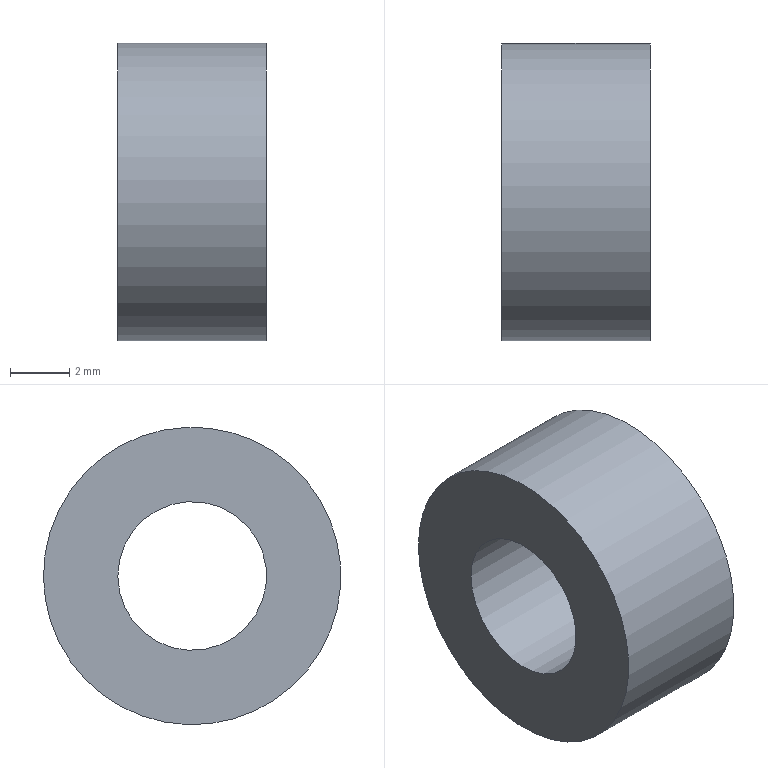Part | STEP file | Dodanie-wyci_gni_cie1_7 | 1 solid | 4 faces | box 5 x 10 x 10 mm | volume 294.524 mm3 | cylinder 2 | plane 2 | commonest cylinder face diameters 5 x1 10 x1
STEP:
#1=CARTESIAN_POINT('',(0.,0.,0.));
#2=DIRECTION('',(0.,0.,1.));
#3=DIRECTION('',(1.,0.,0.));
#4=AXIS2_PLACEMENT_3D('',#1,#2,#3);
#5=CARTESIAN_POINT('',(-60.146,93.261,-75.378));
#6=VERTEX_POINT('',#5);
#7=CARTESIAN_POINT('',(-65.146,93.261,-75.378));
#8=VERTEX_POINT('',#7);
#9=CARTESIAN_POINT('',(-60.146,93.261,-75.378));
#10=DIRECTION('',(-1.,0.,0.));
#11=VECTOR('',#10,1.);
#12=LINE('',#9,#11);
#13=CARTESIAN_POINT('',(-65.146,88.261,-75.356));
#14=DIRECTION('',(1.,0.,0.));
#15=DIRECTION('',(0.,1.,-0.004452));
#16=AXIS2_PLACEMENT_3D('',#13,#14,#15);
#17=CYLINDRICAL_SURFACE('',#16,5.);
#18=CARTESIAN_POINT('',(0.,5.));
#19=DIRECTION('',(0.,-1.));
#20=VECTOR('',#19,1.);
#21=LINE('',#18,#20);
#22=(GEOMETRIC_REPRESENTATION_CONTEXT(2)PARAMETRIC_REPRESENTATION_CONTEXT()REPRESENTATION_CONTEXT('',''));
#23=DEFINITIONAL_REPRESENTATION('',(#21),#22);
#24=PCURVE('',#17,#23);
#25=CARTESIAN_POINT('',(6.283,5.));
#26=DIRECTION('',(0.,-1.));
#27=VECTOR('',#26,1.);
#28=LINE('',#25,#27);
#29=(GEOMETRIC_REPRESENTATION_CONTEXT(2)PARAMETRIC_REPRESENTATION_CONTEXT()REPRESENTATION_CONTEXT('',''));
#30=DEFINITIONAL_REPRESENTATION('',(#28),#29);
#31=PCURVE('',#17,#30);
#32=SEAM_CURVE('',#12,(#24,#31),.PCURVE_S1.);
#33=EDGE_CURVE('',#6,#8,#32,.T.);
#34=ORIENTED_EDGE('',*,*,#33,.T.);
#35=CARTESIAN_POINT('',(-65.146,88.261,-75.356));
#36=DIRECTION('',(1.,0.,0.));
#37=DIRECTION('',(0.,1.,-0.004452));
#38=AXIS2_PLACEMENT_3D('',#35,#36,#37);
#39=CIRCLE('',#38,5.);
#40=CARTESIAN_POINT('',(0.,0.));
#41=DIRECTION('',(1.,0.));
#42=VECTOR('',#41,1.);
#43=LINE('',#40,#42);
#44=(GEOMETRIC_REPRESENTATION_CONTEXT(2)PARAMETRIC_REPRESENTATION_CONTEXT()REPRESENTATION_CONTEXT('',''));
#45=DEFINITIONAL_REPRESENTATION('',(#43),#44);
#46=PCURVE('',#17,#45);
#47=CARTESIAN_POINT('',(-65.146,88.261,-75.356));
#48=DIRECTION('',(-1.,0.,0.));
#49=DIRECTION('',(0.,-1.,0.004452));
#50=AXIS2_PLACEMENT_3D('',#47,#48,#49);
#51=PLANE('',#50);
#52=CARTESIAN_POINT('',(-5.,0.));
#53=CARTESIAN_POINT('',(-5.,8.66));
#54=CARTESIAN_POINT('',(2.5,4.33));
#55=CARTESIAN_POINT('',(10.,0.));
#56=CARTESIAN_POINT('',(2.5,-4.33));
#57=CARTESIAN_POINT('',(-5.,-8.66));
#58=CARTESIAN_POINT('',(-5.,0.));
#59=(BOUNDED_CURVE()B_SPLINE_CURVE(2,(#52,#53,#54,#55,#56,#57,#58),.UNSPECIFIED.,.T.,.F.)B_SPLINE_CURVE_WITH_KNOTS((1,2,2,2,2,1),(-2.094,0.,2.094,4.189,6.283,8.378),.UNSPECIFIED.)CURVE()GEOMETRIC_REPRESENTATION_ITEM()RATIONAL_B_SPLINE_CURVE((1.,0.5,1.,0.5,1.,0.5,1.))REPRESENTATION_ITEM(''));
#60=(GEOMETRIC_REPRESENTATION_CONTEXT(2)PARAMETRIC_REPRESENTATION_CONTEXT()REPRESENTATION_CONTEXT('',''));
#61=DEFINITIONAL_REPRESENTATION('',(#59),#60);
#62=PCURVE('',#51,#61);
#63=SURFACE_CURVE('',#39,(#46,#62),.PCURVE_S1.);
#64=EDGE_CURVE('',#8,#8,#63,.T.);
#65=ORIENTED_EDGE('',*,*,#64,.T.);
#66=ORIENTED_EDGE('',*,*,#33,.F.);
#67=CARTESIAN_POINT('',(-60.146,88.261,-75.356));
#68=DIRECTION('',(-1.,0.,0.));
#69=DIRECTION('',(0.,1.,-0.004452));
#70=AXIS2_PLACEMENT_3D('',#67,#68,#69);
#71=CIRCLE('',#70,5.);
#72=CARTESIAN_POINT('',(6.283,5.));
#73=DIRECTION('',(-1.,0.));
#74=VECTOR('',#73,1.);
#75=LINE('',#72,#74);
#76=(GEOMETRIC_REPRESENTATION_CONTEXT(2)PARAMETRIC_REPRESENTATION_CONTEXT()REPRESENTATION_CONTEXT('',''));
#77=DEFINITIONAL_REPRESENTATION('',(#75),#76);
#78=PCURVE('',#17,#77);
#79=CARTESIAN_POINT('',(-60.146,88.261,-75.356));
#80=DIRECTION('',(-1.,0.,0.));
#81=DIRECTION('',(0.,-1.,0.004452));
#82=AXIS2_PLACEMENT_3D('',#79,#80,#81);
#83=PLANE('',#82);
#84=CARTESIAN_POINT('',(0.,0.));
#85=DIRECTION('',(-1.,0.));
#86=AXIS2_PLACEMENT_2D('',#84,#85);
#87=CIRCLE('',#86,5.);
#88=(GEOMETRIC_REPRESENTATION_CONTEXT(2)PARAMETRIC_REPRESENTATION_CONTEXT()REPRESENTATION_CONTEXT('',''));
#89=DEFINITIONAL_REPRESENTATION('',(#87),#88);
#90=PCURVE('',#83,#89);
#91=SURFACE_CURVE('',#71,(#78,#90),.PCURVE_S1.);
#92=EDGE_CURVE('',#6,#6,#91,.T.);
#93=ORIENTED_EDGE('',*,*,#92,.T.);
#94=EDGE_LOOP('',(#34,#65,#66,#93));
#95=FACE_BOUND('',#94,.T.);
#96=ADVANCED_FACE('',(#95),#17,.T.);
#97=CARTESIAN_POINT('',(-65.146,90.761,-75.367));
#98=VERTEX_POINT('',#97);
#99=CARTESIAN_POINT('',(-65.146,88.261,-75.356));
#100=DIRECTION('',(1.,0.,0.));
#101=DIRECTION('',(0.,1.,-0.004452));
#102=AXIS2_PLACEMENT_3D('',#99,#100,#101);
#103=CIRCLE('',#102,2.5);
#104=CARTESIAN_POINT('',(-65.146,88.261,-75.356));
#105=DIRECTION('',(1.,0.,0.));
#106=DIRECTION('',(0.,1.,-0.004452));
#107=AXIS2_PLACEMENT_3D('',#104,#105,#106);
#108=CYLINDRICAL_SURFACE('',#107,2.5);
#109=CARTESIAN_POINT('',(0.,0.));
#110=DIRECTION('',(1.,0.));
#111=VECTOR('',#110,1.);
#112=LINE('',#109,#111);
#113=(GEOMETRIC_REPRESENTATION_CONTEXT(2)PARAMETRIC_REPRESENTATION_CONTEXT()REPRESENTATION_CONTEXT('',''));
#114=DEFINITIONAL_REPRESENTATION('',(#112),#113);
#115=PCURVE('',#108,#114);
#116=CARTESIAN_POINT('',(-2.5,0.));
#117=CARTESIAN_POINT('',(-2.5,4.33));
#118=CARTESIAN_POINT('',(1.25,2.165));
#119=CARTESIAN_POINT('',(5.,0.));
#120=CARTESIAN_POINT('',(1.25,-2.165));
#121=CARTESIAN_POINT('',(-2.5,-4.33));
#122=CARTESIAN_POINT('',(-2.5,0.));
#123=(BOUNDED_CURVE()B_SPLINE_CURVE(2,(#116,#117,#118,#119,#120,#121,#122),.UNSPECIFIED.,.T.,.F.)B_SPLINE_CURVE_WITH_KNOTS((1,2,2,2,2,1),(-2.094,0.,2.094,4.189,6.283,8.378),.UNSPECIFIED.)CURVE()GEOMETRIC_REPRESENTATION_ITEM()RATIONAL_B_SPLINE_CURVE((1.,0.5,1.,0.5,1.,0.5,1.))REPRESENTATION_ITEM(''));
#124=(GEOMETRIC_REPRESENTATION_CONTEXT(2)PARAMETRIC_REPRESENTATION_CONTEXT()REPRESENTATION_CONTEXT('',''));
#125=DEFINITIONAL_REPRESENTATION('',(#123),#124);
#126=PCURVE('',#51,#125);
#127=SURFACE_CURVE('',#103,(#115,#126),.PCURVE_S1.);
#128=EDGE_CURVE('',#98,#98,#127,.T.);
#129=ORIENTED_EDGE('',*,*,#128,.T.);
#130=CARTESIAN_POINT('',(-60.146,90.761,-75.367));
#131=VERTEX_POINT('',#130);
#132=CARTESIAN_POINT('',(-60.146,90.761,-75.367));
#133=DIRECTION('',(-1.,0.,0.));
#134=VECTOR('',#133,1.);
#135=LINE('',#132,#134);
#136=CARTESIAN_POINT('',(6.283,5.));
#137=DIRECTION('',(0.,-1.));
#138=VECTOR('',#137,1.);
#139=LINE('',#136,#138);
#140=(GEOMETRIC_REPRESENTATION_CONTEXT(2)PARAMETRIC_REPRESENTATION_CONTEXT()REPRESENTATION_CONTEXT('',''));
#141=DEFINITIONAL_REPRESENTATION('',(#139),#140);
#142=PCURVE('',#108,#141);
#143=CARTESIAN_POINT('',(0.,5.));
#144=DIRECTION('',(0.,-1.));
#145=VECTOR('',#144,1.);
#146=LINE('',#143,#145);
#147=(GEOMETRIC_REPRESENTATION_CONTEXT(2)PARAMETRIC_REPRESENTATION_CONTEXT()REPRESENTATION_CONTEXT('',''));
#148=DEFINITIONAL_REPRESENTATION('',(#146),#147);
#149=PCURVE('',#108,#148);
#150=SEAM_CURVE('',#135,(#142,#149),.PCURVE_S1.);
#151=EDGE_CURVE('',#131,#98,#150,.T.);
#152=ORIENTED_EDGE('',*,*,#151,.F.);
#153=CARTESIAN_POINT('',(-60.146,88.261,-75.356));
#154=DIRECTION('',(1.,0.,0.));
#155=DIRECTION('',(0.,1.,-0.004452));
#156=AXIS2_PLACEMENT_3D('',#153,#154,#155);
#157=CIRCLE('',#156,2.5);
#158=CARTESIAN_POINT('',(0.,5.));
#159=DIRECTION('',(1.,0.));
#160=VECTOR('',#159,1.);
#161=LINE('',#158,#160);
#162=(GEOMETRIC_REPRESENTATION_CONTEXT(2)PARAMETRIC_REPRESENTATION_CONTEXT()REPRESENTATION_CONTEXT('',''));
#163=DEFINITIONAL_REPRESENTATION('',(#161),#162);
#164=PCURVE('',#108,#163);
#165=CARTESIAN_POINT('',(-2.5,0.));
#166=CARTESIAN_POINT('',(-2.5,4.33));
#167=CARTESIAN_POINT('',(1.25,2.165));
#168=CARTESIAN_POINT('',(5.,0.));
#169=CARTESIAN_POINT('',(1.25,-2.165));
#170=CARTESIAN_POINT('',(-2.5,-4.33));
#171=CARTESIAN_POINT('',(-2.5,0.));
#172=(BOUNDED_CURVE()B_SPLINE_CURVE(2,(#165,#166,#167,#168,#169,#170,#171),.UNSPECIFIED.,.T.,.F.)B_SPLINE_CURVE_WITH_KNOTS((1,2,2,2,2,1),(-2.094,0.,2.094,4.189,6.283,8.378),.UNSPECIFIED.)CURVE()GEOMETRIC_REPRESENTATION_ITEM()RATIONAL_B_SPLINE_CURVE((1.,0.5,1.,0.5,1.,0.5,1.))REPRESENTATION_ITEM(''));
#173=(GEOMETRIC_REPRESENTATION_CONTEXT(2)PARAMETRIC_REPRESENTATION_CONTEXT()REPRESENTATION_CONTEXT('',''));
#174=DEFINITIONAL_REPRESENTATION('',(#172),#173);
#175=PCURVE('',#83,#174);
#176=SURFACE_CURVE('',#157,(#164,#175),.PCURVE_S1.);
#177=EDGE_CURVE('',#131,#131,#176,.T.);
#178=ORIENTED_EDGE('',*,*,#177,.F.);
#179=ORIENTED_EDGE('',*,*,#151,.T.);
#180=EDGE_LOOP('',(#129,#152,#178,#179));
#181=FACE_BOUND('',#180,.F.);
#182=ADVANCED_FACE('',(#181),#108,.F.);
#183=ORIENTED_EDGE('',*,*,#177,.F.);
#184=EDGE_LOOP('',(#183));
#185=FACE_BOUND('',#184,.T.);
#186=ORIENTED_EDGE('',*,*,#92,.F.);
#187=EDGE_LOOP('',(#186));
#188=FACE_BOUND('',#187,.T.);
#189=ADVANCED_FACE('',(#185,#188),#83,.F.);
#190=ORIENTED_EDGE('',*,*,#128,.T.);
#191=EDGE_LOOP('',(#190));
#192=FACE_BOUND('',#191,.T.);
#193=ORIENTED_EDGE('',*,*,#64,.F.);
#194=EDGE_LOOP('',(#193));
#195=FACE_BOUND('',#194,.T.);
#196=ADVANCED_FACE('',(#192,#195),#51,.T.);
#197=CLOSED_SHELL('',(#96,#182,#189,#196));
#198=MANIFOLD_SOLID_BREP('',#197);
#199=(LENGTH_UNIT()NAMED_UNIT(*)SI_UNIT(.MILLI.,.METRE.));
#200=UNCERTAINTY_MEASURE_WITH_UNIT(LENGTH_MEASURE(0.0000001),#199,'','');
#201=(NAMED_UNIT(*)PLANE_ANGLE_UNIT()SI_UNIT($,.RADIAN.));
#202=(NAMED_UNIT(*)SI_UNIT($,.STERADIAN.)SOLID_ANGLE_UNIT());
#203=(GEOMETRIC_REPRESENTATION_CONTEXT(3)GLOBAL_UNCERTAINTY_ASSIGNED_CONTEXT((#200))GLOBAL_UNIT_ASSIGNED_CONTEXT((#199,#201,#202))REPRESENTATION_CONTEXT('',''));
#204=ADVANCED_BREP_SHAPE_REPRESENTATION('',(#4,#198),#203);